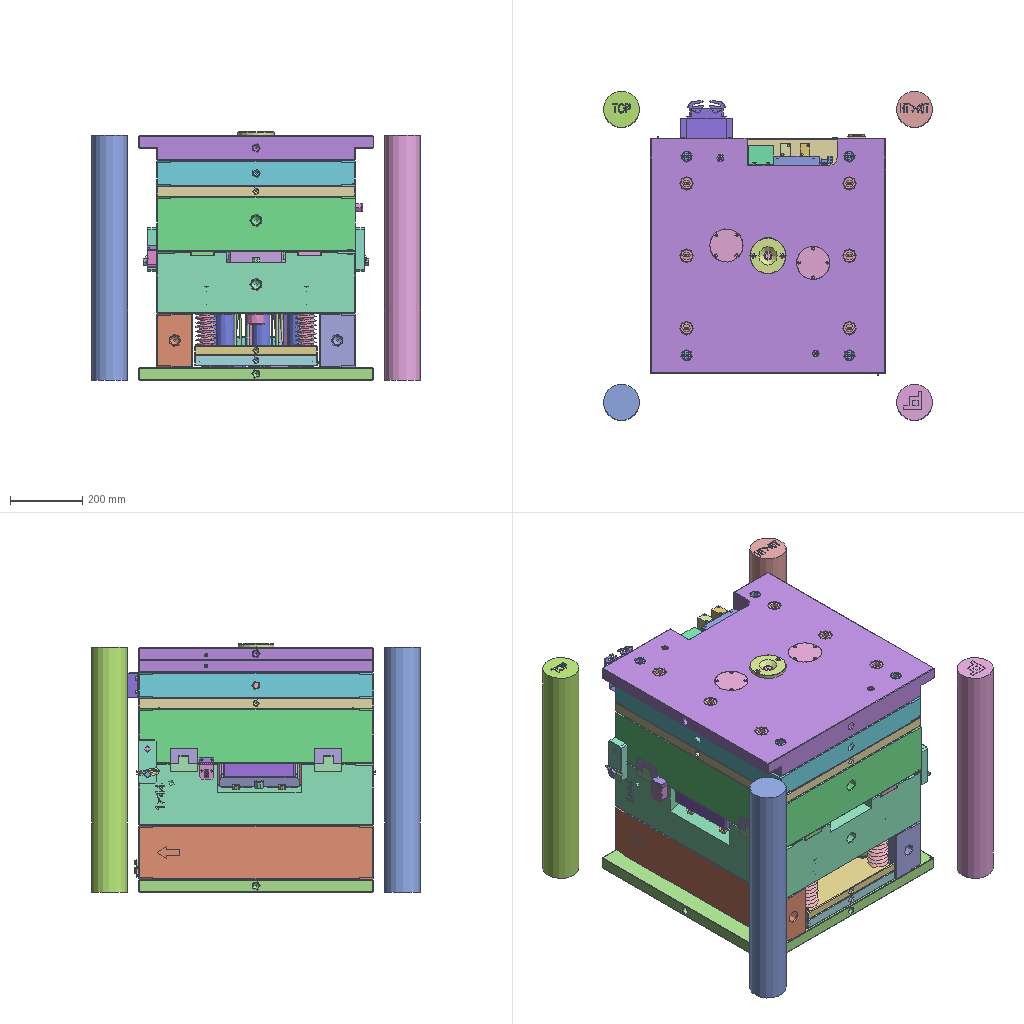Assembly | STEP file | 222 different items | 769 placed | box 910 x 908 x 687 mm
Parts list (item | name | quantity | parent item | size | volume):
1 | Tie Bars 360T | x1 | in 4-Mark_FACET | 910 x 910 x 677 mm | 21266346 mm3
2 | P011002M004-000 | x1 | in 3.1-Core_MODEL | 14.13 x 12.392 x 104.223 mm | 11432 mm3
3 | P011002M001-000 | x1 | in 3.1-Core_MODEL | - | 8732040 mm3
4 | P011002M003-000 | x1 | in 3.1-Core_MODEL | 12.084 x 12.031 x 102.825 mm | 9089 mm3
5 | P011002M005-000 | x1 | in 3.1-Core_MODEL | 67.862 x 16 x 35.33 mm | 24834 mm3
6 | P011002M006-000 | x1 | in 3.1-Core_MODEL | 70.25 x 27 x 35.42 mm | 49386 mm3
7 | P011002M008-000 | x1 | in 3.1-Core_MODEL | 73.5 x 17 x 37.933 mm | 27742 mm3
8 | P011002M009-000 | x1 | in 3.1-Core_MODEL | 73.5 x 19 x 37.504 mm | 38643 mm3
9 | P011002M007-000 | x1 | in 3.1-Core_MODEL | 72.03 x 27.74 x 35.47 mm | 32998 mm3
10 | P011002M002-000 | x1 | in 3.1-Core_MODEL | 110.341 x 214.577 x 105.416 mm | 1490799 mm3
11 | EM10503500 | x12 | in 3.1-Core_MODEL, 3.3.6-Lifter 06_MODEL, 3.3.3-Lifter 03_MODEL, 3.3.4-Lifter 04_MODEL, 3.3.5-Lifter 05_MODEL | 8.5 x 8.5 x 40 mm | 920.076 mm3
12 | EM11211000 | x11 | in 3.1-Core_MODEL | 18 x 18 x 122 mm | 14775 mm3
13 | P011002M012-000 | x1 | in 3.1-Core_MODEL | 16.594 x 32.5 x 39.15 mm | 15176 mm3
14 | EM10606000 | x1 | in 3.1-Core_MODEL | 10 x 10 x 66 mm | 2076 mm3
15 | P011002M013-000 | x1 | in 3.1-Core_MODEL | 17 x 15.5 x 53.228 mm | 4545 mm3
16 | P011002M014-000 | x1 | in 3.1-Core_MODEL | 19 x 16.5 x 58.198 mm | 5006 mm3
17 | P011002M015-000 | x1 | in 3.1-Core_MODEL | 19 x 16.5 x 58.027 mm | 4994 mm3
18 | P011002M011-000 | x1 | in 3.1-Core_MODEL | 10.289 x 8.281 x 94.692 mm | 4991 mm3
19 | P011002M010-000 | x1 | in 3.1-Core_MODEL | 9.465 x 8.201 x 94.193 mm | 4408 mm3
20 | P011002M016-000 | x1 | in 3.1-Core_MODEL | 8.688 x 9.5 x 91.429 mm | 3552 mm3
21 | P011002S001-004 | x1 | in 3.2.1-Slide 01_MODEL | 22 x 82 x 24.22 mm | 33052 mm3
22 | P011002S001-002 | x1 | in 3.2.1-Slide 01_MODEL | 33 x 89.557 x 25 mm | 35725 mm3
23 | P011002S001-003 | x1 | in 3.2.1-Slide 01_MODEL | 22 x 82 x 24.22 mm | 33052 mm3
24 | P011002S001-006 | x1 | in 3.2.1-Slide 01_MODEL | 100 x 50.56 x 14.6 mm | 55263 mm3
25 | P011002S001-007 | x1 | in 3.2.1-Slide 01_MODEL | 20 x 19.153 x 23.411 mm | 6389 mm3
26 | P011002S001-001 | x1 | in 3.2.1-Slide 01_MODEL | 33 x 82.885 x 22 mm | 32044 mm3
27 | P011002S001-000 | x1 | in 3.2.1-Slide 01_MODEL | 120 x 58 x 62.996 mm | 277812 mm3
28 | P011002S001-005 | x1 | in 3.2.1-Slide 01_MODEL | 100 x 15.102 x 35.898 mm | 26958 mm3
29 | EM10802500 | x12 | in 3.2.1-Slide 01_MODEL, 3.2.4-Slide 04_MODEL, 3.3.1-Lifter 01_MODEL, 3.3.2-Lifter 02_MODEL | 13 x 13 x 33 mm | 2154 mm3
30 | EE030603500 | x8 | in 3.2.1-Slide 01_MODEL, 3.2.4-Slide 04_MODEL | 6 x 6 x 37.232 mm | 1919 mm3
31 | SOLID | x58 | in EM10501000 | 8.5 x 8.5 x 15 mm | 429.474 mm3
32 | SOLID | x29 | - | 9.5 x 9.5 x 8 mm | 449.248 mm3
33 | SOLID | x29 | - | 5 x 5 x 12.76 mm | 163.945 mm3
34 | EM10601600 | x39 | in 3.2.1-Slide 01_MODEL, 3.2.2-Slide 02_MODEL, 3.2.3-Slide 03_MODEL, 3.2.4-Slide 04_MODEL, 3.7-Other_MODEL | 10 x 10 x 22 mm | 832.203 mm3
35 | EM10602500 | x20 | in 3.2.1-Slide 01_MODEL, 3.2.2-Slide 02_MODEL, 3.2.3-Slide 03_MODEL, 3.3.1-Lifter 01_MODEL, 3.3.2-Lifter 02_MODEL, 3.3.3-Lifter 03_MODEL, 3.3.5-Lifter 05_MODEL | 10 x 10 x 31 mm | 1087 mm3
36 | EM10803000 | x17 | in 3.2.1-Slide 01_MODEL, 3.2.3-Slide 03_MODEL, 3.2.4-Slide 04_MODEL, 2.2.1-Slide 01_MODEL, 2.2.2-Slide 02_MODEL, 2.2.3-Slide 03_MODEL, 2.2.4-Slide 04_MODEL | 13 x 13 x 38 mm | 2405 mm3
37 | E011204002 | x1 | in 3.2.1-Slide 01_MODEL | - | 1089 mm3
38 | E030603000 | x1 | in 3.2.1-Slide 01_MODEL | 6 x 6 x 32.232 mm | 1637 mm3
39 | P011002S002-000 | x1 | in 3.2.2-Slide 02_MODEL | 70.019 x 220 x 86.547 mm | 835279 mm3
40 | P011002S002-005 | x1 | in 3.2.2-Slide 02_MODEL | 100 x 22 x 65.128 mm | 89552 mm3
41 | P011002S002-002 | x1 | in 3.2.2-Slide 02_MODEL | 103.644 x 32 x 40.64 mm | 72911 mm3
42 | P011002S002-010 | x2 | in 3.2.2-Slide 02_MODEL | 24.439 x 20 x 26.83 mm | 6238 mm3
43 | P011002S002-007 | x1 | in 3.2.2-Slide 02_MODEL | 14.824 x 100 x 40.781 mm | 30059 mm3
44 | P011002S002-003 | x1 | in 3.2.2-Slide 02_MODEL | 94.285 x 31 x 37.408 mm | 61974 mm3
45 | P011002S002-008 | x2 | in 3.2.2-Slide 02_MODEL | 60.486 x 65 x 31.798 mm | 42735 mm3
46 | P011002S002-009 | x1 | in 3.2.2-Slide 02_MODEL | 73.728 x 25 x 55.026 mm | 50035 mm3
47 | P011002S002-004 | x1 | in 3.2.2-Slide 02_MODEL | 100 x 22 x 65.128 mm | 89552 mm3
48 | P011002S002-006 | x1 | in 3.2.2-Slide 02_MODEL | 14.824 x 100 x 40.781 mm | 30059 mm3
49 | P011002S002-001 | x1 | in 3.2.2-Slide 02_MODEL | 113.158 x 33 x 44.092 mm | 87912 mm3
50 | EM10806500 | x2 | in 3.2.2-Slide 02_MODEL | 13 x 13 x 73 mm | 4164 mm3
51 | EE030607000 | x2 | in 3.2.2-Slide 02_MODEL | 6 x 6 x 72.232 mm | 3898 mm3
52 | EM10804500 | x5 | in 3.2.2-Slide 02_MODEL, 2.2.2-Slide 02_MODEL | 13 x 13 x 53 mm | 3159 mm3
53 | EE030606000 | x12 | in 3.2.2-Slide 02_MODEL, 3.2.3-Slide 03_MODEL, 3.3.2-Lifter 02_MODEL | 6 x 6 x 62.232 mm | 3333 mm3
54 | EM10603000 | x6 | in 3.2.2-Slide 02_MODEL, 3.2.4-Slide 04_MODEL, 3.7-Other_MODEL | 10 x 10 x 36 mm | 1228 mm3
55 | EM10804000 | x12 | in 3.2.2-Slide 02_MODEL, 3.2.3-Slide 03_MODEL, 3.7-Other_MODEL, 2.2.3-Slide 03_MODEL | 13 x 13 x 48 mm | 2908 mm3
56 | E011204502 | x6 | in 3.2.2-Slide 02_MODEL, 3.2.3-Slide 03_MODEL, 3.2.4-Slide 04_MODEL | - | 1367 mm3
57 | E030603500 | x6 | in 3.2.2-Slide 02_MODEL, 3.2.3-Slide 03_MODEL, 3.2.4-Slide 04_MODEL | 6 x 6 x 37.232 mm | 1919 mm3
58 | P011002S003-006 | x1 | in 3.2.3-Slide 03_MODEL | 16.561 x 105 x 50.63 mm | 40958 mm3
59 | P011002S003-009 | x1 | in 3.2.3-Slide 03_MODEL | 82.185 x 25 x 53.405 mm | 45412 mm3
60 | P011002S003-005 | x1 | in 3.2.3-Slide 03_MODEL | 100 x 22 x 57.18 mm | 75947 mm3
61 | P011002S003-000 | x1 | in 3.2.3-Slide 03_MODEL | 72.003 x 230 x 92.915 mm | 964495 mm3
62 | P011002S003-007 | x1 | in 3.2.3-Slide 03_MODEL | 16.561 x 105 x 50.63 mm | 40958 mm3
63 | P011002S003-004 | x1 | in 3.2.3-Slide 03_MODEL | 100 x 22 x 57.18 mm | 75947 mm3
64 | P011002S003-001 | x1 | in 3.2.3-Slide 03_MODEL | 113.977 x 32 x 43.155 mm | 84322 mm3
65 | P011002S003-010 | x2 | in 3.2.3-Slide 03_MODEL | 24.439 x 20 x 26.83 mm | 6238 mm3
66 | P011002S003-003 | x1 | in 3.2.3-Slide 03_MODEL | 90.488 x 32 x 36.044 mm | 56970 mm3
67 | P011002S003-008 | x2 | in 3.2.3-Slide 03_MODEL | 60.486 x 82 x 31.798 mm | 54303 mm3
68 | P011002S003-002 | x1 | in 3.2.3-Slide 03_MODEL | 101.347 x 31 x 39.172 mm | 65480 mm3
69 | EM10803500 | x4 | in 3.2.3-Slide 03_MODEL, 3.7-Other_MODEL | 13 x 13 x 43 mm | 2656 mm3
70 | EE030605000 | x2 | in 3.2.3-Slide 03_MODEL | 6 x 6 x 52.232 mm | 2767 mm3
71 | SOLID | x28 | in EM10806000 | 13 x 13 x 68 mm | 3913 mm3
72 | SOLID | x14 | - | 8 x 8 x 21.416 mm | 734.263 mm3
73 | SOLID | x14 | - | 14 x 14 x 55 mm | 4312 mm3
74 | P011002S004-003 | x1 | in 3.2.4-Slide 04_MODEL | 22 x 90 x 22 mm | 37795 mm3
75 | P011002S004-005 | x1 | in 3.2.4-Slide 04_MODEL | 140 x 15.102 x 35.898 mm | 37708 mm3
76 | P011002S004-004 | x1 | in 3.2.4-Slide 04_MODEL | 22 x 90 x 22 mm | 37795 mm3
77 | P011002S004-002 | x1 | in 3.2.4-Slide 04_MODEL | 26 x 79.009 x 22.435 mm | 34276 mm3
78 | P011002S004-000 | x1 | in 3.2.4-Slide 04_MODEL | 162 x 60 x 77 mm | 547857 mm3
79 | P011002S004-007 | x1 | in 3.2.4-Slide 04_MODEL | 20 x 18 x 25 mm | 7143 mm3
80 | P011002S004-001 | x1 | in 3.2.4-Slide 04_MODEL | 29 x 101.051 x 22.958 mm | 42473 mm3
81 | P011002S004-006 | x1 | in 3.2.4-Slide 04_MODEL | 142 x 55 x 12 mm | 88183 mm3
82 | P011002L006-000 | x1 | in 3.3.6-Lifter 06_MODEL | 25 x 8.891 x 318.622 mm | 57302 mm3
83 | P011002L001-000 | x1 | in 3.3.1-Lifter 01_MODEL | 38.903 x 161.923 x 102.441 mm | 296499 mm3
84 | P011002L001-005 | x4 | in 3.3.1-Lifter 01_MODEL | 29.573 x 4.8 x 27.272 mm | 1761 mm3
85 | P011002L001-004 | x2 | in 3.3.1-Lifter 01_MODEL | 36.818 x 34.998 x 27.476 mm | 15941 mm3
86 | P011002L001-003 | x2 | in 3.3.1-Lifter 01_MODEL | 75 x 68 x 55 mm | 144794 mm3
87 | P011002L001-001 | x2 | in 3.3.1-Lifter 01_MODEL | 43.362 x 16 x 275.795 mm | 48038 mm3
88 | P011002L001-002 | x2 | in 3.3.1-Lifter 01_MODEL | 55 x 25 x 20 mm | 20325 mm3
89 | EE030606500 | x8 | in 3.3.1-Lifter 01_MODEL | 6 x 6 x 67.232 mm | 3615 mm3
90 | SOLID | x8 | in EE060800001 | 12.7 x 12.7 x 2 mm | 149.833 mm3
91 | P011002L001-007 | x1 | in 3.3.1-Lifter 01_MODEL | 8.861 x 29.5 x 8.749 mm | 1779 mm3
92 | P011002L001-006 | x1 | in 3.3.1-Lifter 01_MODEL | 8.861 x 29.5 x 8.749 mm | 1779 mm3
93 | EM40301200 | x4 | in 3.3.1-Lifter 01_MODEL, 3.3.2-Lifter 02_MODEL | 6.84 x 6.84 x 16.272 mm | 238.801 mm3
94 | P011002L002-000 | x1 | in 3.3.2-Lifter 02_MODEL | 38.575 x 161.92 x 99.169 mm | 274542 mm3
95 | P011002L002-002 | x2 | in 3.3.2-Lifter 02_MODEL | 55 x 25 x 20 mm | 20325 mm3
96 | P011002L002-003 | x2 | in 3.3.2-Lifter 02_MODEL | 75 x 68 x 50 mm | 123835 mm3
97 | P011002L002-004 | x2 | in 3.3.2-Lifter 02_MODEL | 36.818 x 34.998 x 27.476 mm | 15941 mm3
98 | P011002L002-005 | x4 | in 3.3.2-Lifter 02_MODEL | 27.634 x 4.8 x 24.553 mm | 1761 mm3
99 | P011002L002-001 | x2 | in 3.3.2-Lifter 02_MODEL | 43.362 x 16 x 275.795 mm | 48288 mm3
100 | EM10805500 | x8 | in 3.3.2-Lifter 02_MODEL | 13 x 13 x 63 mm | 3662 mm3
101 | P011002L002-007 | x1 | in 3.3.2-Lifter 02_MODEL | 8.861 x 29.5 x 8.749 mm | 1779 mm3
102 | P011002L002-006 | x1 | in 3.3.2-Lifter 02_MODEL | 8.861 x 29.5 x 8.749 mm | 1779 mm3
103 | P011002L003-000 | x1 | in 3.3.3-Lifter 03_MODEL | 25 x 7.502 x 312.004 mm | 56592 mm3
104 | P011002L003-001 | x1 | in 3.3.3-Lifter 03_MODEL | 80 x 45 x 20 mm | 57856 mm3
105 | P011002L004-000 | x1 | in 3.3.4-Lifter 04_MODEL | 25 x 7.502 x 311.018 mm | 56283 mm3
106 | P011002L005-000 | x1 | in 3.3.5-Lifter 05_MODEL | 25 x 7.509 x 319.656 mm | 57786 mm3
107 | P011002L005-001 | x1 | in 3.3.5-Lifter 05_MODEL | 100 x 40 x 20 mm | 68887 mm3
108 | 3.4-Cooling System | x2 | in 3-Core Side ASM_MODEL | - | -
109 | E108-07-310 | x1 | in 3.5-Ejector System_TRUE | 13 x 16.5 x 303.697 mm | 15889 mm3
110 | E106-16-310 | x1 | in 3.5-Ejector System_TRUE | 10 x 13 x 301.324 mm | 8818 mm3
111 | E108-10-310 | x1 | in 3.5-Ejector System_TRUE | 13 x 16.5 x 302.023 mm | 15811 mm3
112 | E105-28-315 | x1 | in 3.5-Ejector System_TRUE | 9 x 12 x 309.813 mm | 6362 mm3
113 | E108-12-310 | x1 | in 3.5-Ejector System_TRUE | 13 x 16.5 x 306.86 mm | 16065 mm3
114 | E108-11-315 | x1 | in 3.5-Ejector System_TRUE | 13 x 16.5 x 310.586 mm | 16274 mm3
115 | E108-05-325 | x1 | in 3.5-Ejector System_TRUE | 13 x 16.5 x 321.213 mm | 16796 mm3
116 | E108-03-320 | x1 | in 3.5-Ejector System_TRUE | 13 x 16.5 x 312.703 mm | 16360 mm3
117 | E106-25-315 | x1 | in 3.5-Ejector System_TRUE | 10 x 13 x 312.463 mm | 9128 mm3
118 | E108-15-310 | x1 | in 3.5-Ejector System_TRUE | 13 x 16.5 x 280 mm | 14461 mm3
119 | E106-18-310 | x1 | in 3.5-Ejector System_TRUE | 10 x 13 x 299.38 mm | 8763 mm3
120 | E106-23-315 | x1 | in 3.5-Ejector System_TRUE | 10 x 13 x 307.684 mm | 8994 mm3
121 | E108-14-310 | x1 | in 3.5-Ejector System_TRUE | 13 x 16.5 x 280 mm | 14461 mm3
122 | E106-13-315 | x1 | in 3.5-Ejector System_TRUE | 10 x 13 x 309.676 mm | 9056 mm3
123 | E106-17-310 | x1 | in 3.5-Ejector System_TRUE | 10 x 13 x 302.496 mm | 8853 mm3
124 | E108-04-325 | x1 | in 3.5-Ejector System_TRUE | 13 x 16.5 x 322.523 mm | 16862 mm3
125 | E108-08-310 | x1 | in 3.5-Ejector System_TRUE | 13 x 16.5 x 302.869 mm | 15847 mm3
126 | E106-20-315 | x1 | in 3.5-Ejector System_TRUE | 10 x 13 x 307.336 mm | 8991 mm3
127 | E106-26-325 | x1 | in 3.5-Ejector System_TRUE | 10 x 13 x 318.085 mm | 9301 mm3
128 | E108-06-310 | x1 | in 3.5-Ejector System_TRUE | 13 x 16.5 x 302.992 mm | 15844 mm3
129 | E108-09-310 | x1 | in 3.5-Ejector System_TRUE | 13 x 16.5 x 301.993 mm | 15803 mm3
130 | E105-29-315 | x1 | in 3.5-Ejector System_TRUE | 9 x 12 x 311.151 mm | 6392 mm3
131 | E106-21-315 | x1 | in 3.5-Ejector System_TRUE | 10 x 13 x 308.066 mm | 9009 mm3
132 | E105-27-315 | x1 | in 3.5-Ejector System_TRUE | 9 x 12 x 304.744 mm | 6258 mm3
133 | E105-30-315 | x1 | in 3.5-Ejector System_TRUE | 9 x 12 x 311.08 mm | 6391 mm3
134 | E108-1-312 | x1 | in 3.5-Ejector System_TRUE | 13 x 16.5 x 290 mm | 14963 mm3
135 | E105-19-315 | x1 | in 3.5-Ejector System_TRUE | 9 x 12 x 309.26 mm | 6349 mm3
136 | 3.6-Runner System | x1 | in 3-Core Side ASM_MODEL | - | -
137 | P011002NM05-000 | x1 | in 3.7-Other_MODEL | 65 x 100 x 12 mm | 66526 mm3
138 | P011002NM02-000 | x2 | in 3.7-Other_MODEL | 50 x 85 x 12 mm | 47864 mm3
139 | P011002NM01-000 | x2 | in 3.7-Other_MODEL | 84 x 80 x 12 mm | 69166 mm3
140 | P011002NM03-000 | x2 | in 3.7-Other_MODEL | 35 x 70 x 12 mm | 28000 mm3
141 | P011002NM04-000 | x1 | in 3.7-Other_MODEL | 65 x 100 x 12 mm | 66526 mm3
142 | P011002NM06-000 | x1 | in 3.7-Other_MODEL | 31 x 77 x 69 mm | 123856 mm3
143 | P011002NM07-000 | x1 | in 3.7-Other_MODEL | 87 x 31 x 69 mm | 142784 mm3
144 | P011002NM08-000 | x1 | in 3.7-Other_MODEL | 88 x 31 x 69 mm | 144711 mm3
145 | P011002NM09-000 | x1 | in 3.7-Other_MODEL | 31 x 57 x 69 mm | 94738 mm3
146 | EM11007500 | x7 | in 3.7-Other_MODEL | 16 x 16 x 85 mm | 7551 mm3
147 | P011002NM10-000 | x3 | in 3.7-Other_MODEL | 35 x 35 x 38 mm | 32907 mm3
148 | P011002NM12-000 | x7 | in 3.7-Other_MODEL | 50 x 50 x 150 mm | 291723 mm3
149 | P011002NM11-000 | x2 | in 3.7-Other_MODEL | 40 x 40 x 150 mm | 185820 mm3
150 | P011002NM13-000 | x2 | in 3.7-Other_MODEL | 50 x 50 x 30 mm | 55572 mm3
151 | P011002NM14-000 | x1 | in 3.7-Other_MODEL | 150 x 50 x 25 mm | 168344 mm3
152 | P011002NM16-000 | x1 | in 3.7-Other_MODEL | 50 x 5 x 49 mm | 10135 mm3
153 | P011002NM15-000 | x1 | in 3.7-Other_MODEL | 30 x 5 x 50 mm | 7166 mm3
154 | E112002500 | x4 | in 3.7-Other_MODEL | 20 x 20 x 20 mm | 6268 mm3
155 | E016017503 | x4 | in 3.7-Other_MODEL | - | 163409 mm3
156 | PH15012004 | x2 | in 3.7-Other_MODEL | 65.87 x 120 x 90.403 mm | 187828 mm3
157 | EM11204000 | x9 | in 3.7-Other_MODEL | 18 x 18 x 52 mm | 6858 mm3
158 | EM10301400 | x2 | in 3.7-Other_MODEL | 5 x 5 x 17 mm | 149.174 mm3
159 | EM10401000 | x2 | in 3.7-Other_MODEL | 7 x 7 x 14 mm | 262.339 mm3
160 | EN80200001 | x1 | in 3.7-Other_MODEL | 21 x 20.3 x 18.187 mm | 1904 mm3
161 | E050000001 | x1 | in 3.7-Other_MODEL | 26.859 x 11 x 37.801 mm | 4792 mm3
162 | EM10601400 | x2 | in 3.7-Other_MODEL | 10 x 10 x 20 mm | 775.654 mm3
163 | E042000001 | x1 | in 3.7-Other_MODEL | 38 x 60 x 38.607 mm | 56849 mm3
164 | D17XH8Xd12XA6XB8X310LXN180 | x1 | in 3.7-Other_MODEL | 15.5 x 17 x 309.851 mm | 27016 mm3
165 | P011002B001-000 | x1 | in 3.8-Mold base_MODEL | - | 41496641 mm3
166 | P011002C002-000 | x2 | in P011002C001-000_MODEL, 3.8-Mold base_MODEL | 100 x 650 x 150 mm | 9316840 mm3
167 | SOLID | x1 | in P011002C001-000_MODEL | 100 x 650 x 150 mm | 9243091 mm3
168 | P011002B004-000 | x1 | in 3.8-Mold base_MODEL | 650 x 650 x 35 mm | 13284442 mm3
169 | RP-D30-287L | x4 | in 3.8-Mold base_MODEL | 36 x 36 x 287 mm | 205979 mm3
170 | P011002B003-000 | x1 | in 3.8-Mold base_MODEL | 340 x 650 x 30 mm | 5385169 mm3
171 | P011002B002-000 | x1 | in 3.8-Mold base_MODEL | 340 x 650 x 25 mm | 4617723 mm3
172 | LKM-Top Locks-TOP_75-B | x4 | in 3.8-Mold base_MODEL | 30 x 75 x 51.5 mm | 60575 mm3
173 | DP20-1 | x8 | in 3.8-Mold base_MODEL | 20 x 20 x 71.774 mm | 40454 mm3
174 | M24-1 | x6 | in 3.8-Mold base_MODEL | 36 x 36 x 214 mm | 107145 mm3
175 | M16-2 | x8 | in 3.8-Mold base_MODEL | 24 x 24 x 56 mm | 13524 mm3
176 | GP50 | x4 | in 3.8-Mold base_MODEL | 58 x 58 x 310 mm | 612293 mm3
177 | EGP | x4 | in 3.8-Mold base_MODEL | 45 x 45 x 220 mm | 186041 mm3
178 | STP | x14 | in 3.8-Mold base_MODEL | 28 x 28 x 12.4 mm | 3112 mm3
179 | M12-1 | x8 | in 3.8-Mold base_MODEL | 18 x 18 x 47 mm | 6292 mm3
180 | P011002F001-000 | x1 | in 2.1-Cavity_MODEL | - | 7659861 mm3
181 | EM11207000 | x8 | in 2.1-Cavity_MODEL | 18 x 18 x 82 mm | 10251 mm3
182 | P011002S001-008 | x1 | in 2.2.1-Slide 01_MODEL | 25 x 35.334 x 83.861 mm | 28077 mm3
183 | P011002S001-009 | x1 | in 2.2.1-Slide 01_MODEL | 100 x 85 x 70 mm | 323771 mm3
184 | EM10807500 | x2 | in 2.2.1-Slide 01_MODEL | 13 x 13 x 83 mm | 4667 mm3
185 | P011002S002-011 | x2 | in 2.2.2-Slide 02_MODEL | 34.904 x 25 x 99.124 mm | 32836 mm3
186 | P011002S002-012 | x1 | in 2.2.2-Slide 02_MODEL | 110 x 190 x 78 mm | 738525 mm3
187 | P011002S003-011 | x2 | in 2.2.3-Slide 03_MODEL | 36.296 x 25 x 109.027 mm | 35448 mm3
188 | P011002S003-012 | x1 | in 2.2.3-Slide 03_MODEL | 110 x 200 x 90 mm | 805824 mm3
189 | P011002S004-008 | x2 | in 2.2.4-Slide 04_MODEL | 20 x 32.087 x 88.754 mm | 18799 mm3
190 | P011002S004-009 | x1 | in 2.2.4-Slide 04_MODEL | 135 x 40 x 25 mm | 110970 mm3
191 | 2.3-Lifter | x1 | in 2-Cavity Side ASM_MODEL | - | -
192 | SOLID | x22 | in EM3380000 | 16.662 x 16.662 x 12.01 mm | 2091 mm3
193 | SOLID | x11 | - | 16.662 x 16.662 x 12.01 mm | 1384 mm3
194 | EN53801200 | x4 | in CO-FC-01_MODEL, CO-FC-02_MODEL | 22 x 24.249 x 32.01 mm | 7856 mm3
195 | EC21600001 | x4 | in CO-FC-01_MODEL, CO-FC-02_MODEL | 22.4 x 22.4 x 1.8 mm | 613.838 mm3
196 | SOLID | x1 | in CO-FC-01_MODEL | 356 x 182.01 x 78 mm | 174730 mm3
197 | EC31200008 | x1 | in CO-FC-02_MODEL | 12 x 12 x 12 mm | 1282 mm3
198 | SOLID | x1 | in CO-FC-02_MODEL | 440 x 197.312 x 76 mm | 258377 mm3
199 | 2.5-Ejector System | x1 | in 2-Cavity Side ASM_MODEL | - | -
200 | EM31800001 | x4 | in 2.6-Runner System_MODEL | 9.728 x 9.728 x 8.365 mm | 484.697 mm3
201 | EM10503000 | x4 | in 2.6-Runner System_MODEL | 9.5 x 9.5 x 40.261 mm | 1873 mm3
202 | M10600800 | x4 | in 2.6-Runner System_MODEL | 10 x 10 x 24.812 mm | 985.086 mm3
203 | COMPOUND | x1 | in 2.6-Runner System_MODEL | 514.266 x 513.429 x 330.33 mm | 7966584 mm3
204 | P011002NF02-000 | x3 | in 2.7-Other_MODEL | 80 x 31 x 84 mm | 154459 mm3
205 | P011002NF03-000 | x1 | in 2.7-Other_MODEL | 31 x 60 x 84 mm | 108643 mm3
206 | EM11009000 | x8 | in 2.7-Other_MODEL | 16 x 16 x 100 mm | 8729 mm3
207 | P011002NF01-000 | x1 | in 2.7-Other_MODEL | 100 x 100 x 18 mm | 119839 mm3
208 | EM10802000 | x2 | in 2.7-Other_MODEL | 13 x 13 x 28 mm | 1902 mm3
209 | EM40500800 | x6 | in 2.7-Other_MODEL | 11.4 x 11.4 x 17.76 mm | 658.01 mm3
210 | P011002NF05-000 | x1 | in 2.7-Other_MODEL | 75 x 192.5 x 5 mm | 70540 mm3
211 | P011002NF04-000 | x1 | in 2.7-Other_MODEL | 190 x 75 x 5 mm | 70407 mm3
212 | P011002A003-000 | x1 | in 2.8-Mold base_MODEL | 550 x 650 x 70 mm | 18968143 mm3
213 | P011002A002-000 | x1 | in 2.8-Mold base_MODEL | 550 x 650 x 30 mm | 10420877 mm3
214 | P011002A004-000 | x1 | in 2.8-Mold base_MODEL | 650 x 650 x 70 mm | 24694977 mm3
215 | P011002A001-000 | x1 | in 2.8-Mold base_MODEL | 550 x 650 x 150 mm | 35811112 mm3
216 | M24-2 | x6 | in 2.8-Mold base_MODEL | 36 x 36 x 204 mm | 102621 mm3
217 | M20-1 | x4 | in 2.8-Mold base_MODEL | 30 x 30 x 100 mm | 36177 mm3
218 | M16-1 | x4 | in 2.8-Mold base_MODEL | 24 x 24 x 96 mm | 21566 mm3
219 | DP20X210 | x2 | in 2.8-Mold base_MODEL | 20 x 20 x 210 mm | 65178 mm3
220 | LKM-Top Locks-TOP_75-A | x4 | in 2.8-Mold base_MODEL | 30 x 75 x 51.5 mm | 70556 mm3
221 | GB-D50-150L | x4 | in 2.8-Mold base_MODEL | 76 x 76 x 150 mm | 293063 mm3
222 | 20110925@CORE-RH | x1 | in 1-Product_FACET | 186.272 x 292.181 x 109.099 mm | 237694 mm3
Placements (level | parent | child | x y z in mm | rotation matrix by rows), first 285 of 914 lines:
1 | subassembly 2 | 4-Mark_FACET | 0.0 0.0 0.0 | 1 0 0 0 1 0 0 0 1
2 | 4-Mark_FACET | Tie Bars 360T | 0.0 0.0 0.0 | 1 0 0 0 1 0 0 0 1
1 | subassembly 2 | 3-Core Side ASM_MODEL | 0.0 0.0 0.0 | 1 0 0 0 1 0 0 0 1
2 | 3-Core Side ASM_MODEL | 3.1-Core_MODEL | 0.0 0.0 0.0 | 1 0 0 0 1 0 0 0 1
3 | 3.1-Core_MODEL | P011002M004-000 | 0.0 0.0 0.0 | 1 0 0 0 1 0 0 0 1
3 | 3.1-Core_MODEL | P011002M001-000 | 0.0 0.0 0.0 | 1 0 0 0 1 0 0 0 1
3 | 3.1-Core_MODEL | P011002M003-000 | 0.0 0.0 0.0 | 1 0 0 0 1 0 0 0 1
3 | 3.1-Core_MODEL | P011002M005-000 | 0.0 0.0 0.0 | 1 0 0 0 1 0 0 0 1
3 | 3.1-Core_MODEL | P011002M006-000 | 0.0 0.0 0.0 | 1 0 0 0 1 0 0 0 1
3 | 3.1-Core_MODEL | P011002M008-000 | 0.0 0.0 0.0 | 1 0 0 0 1 0 0 0 1
3 | 3.1-Core_MODEL | P011002M009-000 | 0.0 0.0 0.0 | 1 0 0 0 1 0 0 0 1
3 | 3.1-Core_MODEL | P011002M007-000 | 0.0 0.0 0.0 | 1 0 0 0 1 0 0 0 1
3 | 3.1-Core_MODEL | P011002M002-000 | 0.0 0.0 0.0 | 1 0 0 0 1 0 0 0 1
3 | 3.1-Core_MODEL | EM10503500 | -129.932 40.02 37.0 | 1 0 0 0 1 0 0 0 1
3 | 3.1-Core_MODEL | EM10503500 | 107.019 -21.406 27.0 | 1 0 0 0 1 0 0 0 1
3 | 3.1-Core_MODEL | EM10503500 | 144.019 -21.406 27.0 | 1 0 0 0 1 0 0 0 1
3 | 3.1-Core_MODEL | EM10503500 | -108.932 42.02 37.0 | 1 0 0 0 1 0 0 0 1
3 | 3.1-Core_MODEL | EM11211000 | -15.0 12.0 -151.0 | -1 0 0 0 1 0 0 0 -1
3 | 3.1-Core_MODEL | EM11211000 | 145.0 -180.0 -151.0 | -1 0 0 0 1 0 0 0 -1
3 | 3.1-Core_MODEL | EM11211000 | 20.0 -38.0 -151.0 | -1 0 0 0 1 0 0 0 -1
3 | 3.1-Core_MODEL | EM11211000 | -15.0 -68.0 -151.0 | -1 0 0 0 1 0 0 0 -1
3 | 3.1-Core_MODEL | EM11211000 | -145.0 180.0 -151.0 | -1 0 0 0 1 0 0 0 -1
3 | 3.1-Core_MODEL | EM11211000 | 20.0 52.0 -151.0 | -1 0 0 0 1 0 0 0 -1
3 | 3.1-Core_MODEL | EM11211000 | -145.0 20.0 -151.0 | -1 0 0 0 1 0 0 0 -1
3 | 3.1-Core_MODEL | EM11211000 | 145.0 45.0 -151.0 | -1 0 0 0 1 0 0 0 -1
3 | 3.1-Core_MODEL | EM11211000 | 145.0 180.0 -151.0 | -1 0 0 0 1 0 0 0 -1
3 | 3.1-Core_MODEL | EM11211000 | -15.0 77.0 -151.0 | -1 0 0 0 1 0 0 0 -1
3 | 3.1-Core_MODEL | EM11211000 | -145.0 -180.0 -151.0 | -1 0 0 0 1 0 0 0 -1
3 | 3.1-Core_MODEL | P011002M012-000 | 0.0 0.0 0.0 | 1 0 0 0 1 0 0 0 1
3 | 3.1-Core_MODEL | EM10606000 | -70.0 -4.5 -48.0 | -1 0 0 0 1 0 0 0 -1
3 | 3.1-Core_MODEL | P011002M013-000 | 0.0 0.0 0.0 | 1 0 0 0 1 0 0 0 1
3 | 3.1-Core_MODEL | P011002M014-000 | 0.0 0.0 0.0 | 1 0 0 0 1 0 0 0 1
3 | 3.1-Core_MODEL | P011002M015-000 | 0.0 0.0 0.0 | 1 0 0 0 1 0 0 0 1
3 | 3.1-Core_MODEL | P011002M011-000 | 0.0 0.0 0.0 | 1 0 0 0 1 0 0 0 1
3 | 3.1-Core_MODEL | P011002M010-000 | 0.0 0.0 0.0 | 1 0 0 0 1 0 0 0 1
3 | 3.1-Core_MODEL | P011002M016-000 | 0.0 0.0 0.0 | 1 0 0 0 1 0 0 0 1
2 | 3-Core Side ASM_MODEL | 3.2-Slide_MODEL | 0.0 0.0 0.0 | 1 0 0 0 1 0 0 0 1
3 | 3.2-Slide_MODEL | 3.2.1-Slide 01_MODEL | 0.0 0.0 0.0 | 1 0 0 0 1 0 0 0 1
4 | 3.2.1-Slide 01_MODEL | P011002S001-004 | 0.0 0.0 0.0 | 1 0 0 0 1 0 0 0 1
4 | 3.2.1-Slide 01_MODEL | P011002S001-002 | 0.0 0.0 0.0 | 1 0 0 0 1 0 0 0 1
4 | 3.2.1-Slide 01_MODEL | P011002S001-003 | 0.0 0.0 0.0 | 1 0 0 0 1 0 0 0 1
4 | 3.2.1-Slide 01_MODEL | P011002S001-006 | 0.0 0.0 0.0 | 1 0 0 0 1 0 0 0 1
4 | 3.2.1-Slide 01_MODEL | P011002S001-007 | 0.0 0.0 0.0 | 1 0 0 0 1 0 0 0 1
4 | 3.2.1-Slide 01_MODEL | P011002S001-001 | 0.0 0.0 0.0 | 1 0 0 0 1 0 0 0 1
4 | 3.2.1-Slide 01_MODEL | P011002S001-000 | 0.0 0.0 0.0 | 1 0 0 0 1 0 0 0 1
4 | 3.2.1-Slide 01_MODEL | P011002S001-005 | 0.0 0.0 0.0 | 1 0 0 0 1 0 0 0 1
4 | 3.2.1-Slide 01_MODEL | EM10802500 | -67.5 212.0 19.0 | 1 0 0 0 1 0 0 0 1
4 | 3.2.1-Slide 01_MODEL | EM10802500 | 66.5 212.0 19.0 | 1 0 0 0 1 0 0 0 1
4 | 3.2.1-Slide 01_MODEL | EE030603500 | 66.5 230.0 19.0 | 1 0 0 0 1 0 0 0 1
4 | 3.2.1-Slide 01_MODEL | EM10802500 | -67.5 268.0 19.0 | 1 0 0 0 1 0 0 0 1
4 | 3.2.1-Slide 01_MODEL | EE030603500 | -67.5 249.0 19.0 | 1 0 0 0 1 0 0 0 1
4 | 3.2.1-Slide 01_MODEL | EE030603500 | -67.5 230.0 19.0 | 1 0 0 0 1 0 0 0 1
4 | 3.2.1-Slide 01_MODEL | EM10802500 | 66.5 268.0 19.0 | 1 0 0 0 1 0 0 0 1
4 | 3.2.1-Slide 01_MODEL | EE030603500 | 66.5 249.0 19.0 | 1 0 0 0 1 0 0 0 1
4 | 3.2.1-Slide 01_MODEL | EM10501000 | 34.5 253.791 26.161 | 0 1 0 -0.2079 0 0.9781 0.9781 0 0.2079
5 | EM10501000 | SOLID | 0.0 0.0 0.0 | 1 0 0 0 1 0 0 0 1
5 | EM10501000 | subassembly 1 | 0.0 0.0 0.0 | 1 0 0 0 1 0 0 0 1
6 | subassembly 1 | SOLID | 0.0 0.0 0.0 | 1 0 0 0 1 0 0 0 1
6 | subassembly 1 | SOLID | 0.0 0.0 0.0 | 1 0 0 0 1 0 0 0 1
6 | subassembly 1 | SOLID | 0.0 0.0 0.0 | 1 0 0 0 1 0 0 0 1
4 | 3.2.1-Slide 01_MODEL | EM10501000 | -35.5 253.791 26.161 | 0 1 0 -0.2079 0 0.9781 0.9781 0 0.2079
5 | EM10501000 | SOLID | 0.0 0.0 0.0 | 1 0 0 0 1 0 0 0 1
5 | EM10501000 | subassembly 1 | 0.0 0.0 0.0 | 1 0 0 0 1 0 0 0 1
6 | subassembly 1 | SOLID | 0.0 0.0 0.0 | 1 0 0 0 1 0 0 0 1
6 | subassembly 1 | SOLID | 0.0 0.0 0.0 | 1 0 0 0 1 0 0 0 1
6 | subassembly 1 | SOLID | 0.0 0.0 0.0 | 1 0 0 0 1 0 0 0 1
4 | 3.2.1-Slide 01_MODEL | EM10601600 | -35.5 255.167 -11.891 | 0 -1 0 0.9986 0 0.05234 -0.05234 0 0.9986
4 | 3.2.1-Slide 01_MODEL | EM10601600 | -35.5 225.208 -10.321 | 0 -1 0 0.9986 0 0.05234 -0.05234 0 0.9986
4 | 3.2.1-Slide 01_MODEL | EM10601600 | 34.5 225.208 -10.321 | 0 -1 0 0.9986 0 0.05234 -0.05234 0 0.9986
4 | 3.2.1-Slide 01_MODEL | EM10601600 | 34.5 255.167 -11.891 | 0 -1 0 0.9986 0 0.05234 -0.05234 0 0.9986
4 | 3.2.1-Slide 01_MODEL | EM10602500 | -0.5 274.69 -2.4 | 0 -1 0 0.9986 0 0.05234 -0.05234 0 0.9986
4 | 3.2.1-Slide 01_MODEL | EM10803000 | -33.5 210.0 50.0 | 0 -1 0 0.9986 0 0.05234 -0.05234 0 0.9986
4 | 3.2.1-Slide 01_MODEL | EM10803000 | 31.5 210.0 46.0 | 0 -1 0 0.9986 0 0.05234 -0.05234 0 0.9986
4 | 3.2.1-Slide 01_MODEL | E011204002 | -0.5 214.979 0.215 | 0 1 0 -0.05234 0 -0.9986 -0.9986 0 0.05234
4 | 3.2.1-Slide 01_MODEL | E030603000 | -0.5 212.982 0.3196 | 0 1 0 0.05234 0 0.9986 0.9986 0 -0.05234
3 | 3.2-Slide_MODEL | 3.2.2-Slide 02_MODEL | 0.0 0.0 0.0 | 1 0 0 0 1 0 0 0 1
4 | 3.2.2-Slide 02_MODEL | P011002S002-000 | 0.0 0.0 0.0 | 1 0 0 0 1 0 0 0 1
4 | 3.2.2-Slide 02_MODEL | P011002S002-005 | 0.0 0.0 0.0 | 1 0 0 0 1 0 0 0 1
4 | 3.2.2-Slide 02_MODEL | P011002S002-002 | 0.0 0.0 0.0 | 1 0 0 0 1 0 0 0 1
4 | 3.2.2-Slide 02_MODEL | P011002S002-010 | 0.0 0.0 0.0 | 1 0 0 0 1 0 0 0 1
4 | 3.2.2-Slide 02_MODEL | P011002S002-007 | 0.0 0.0 0.0 | 1 0 0 0 1 0 0 0 1
4 | 3.2.2-Slide 02_MODEL | P011002S002-003 | 0.0 0.0 0.0 | 1 0 0 0 1 0 0 0 1
4 | 3.2.2-Slide 02_MODEL | P011002S002-008 | 0.0 -132.5 0.0 | 1 0 0 0 1 0 0 0 1
4 | 3.2.2-Slide 02_MODEL | P011002S002-009 | 0.0 0.0 0.0 | 1 0 0 0 1 0 0 0 1
4 | 3.2.2-Slide 02_MODEL | P011002S002-008 | 0.0 0.0 0.0 | 1 0 0 0 1 0 0 0 1
4 | 3.2.2-Slide 02_MODEL | P011002S002-004 | 0.0 0.0 0.0 | 1 0 0 0 1 0 0 0 1
4 | 3.2.2-Slide 02_MODEL | P011002S002-010 | 0.0 -132.5 0.0 | 1 0 0 0 1 0 0 0 1
4 | 3.2.2-Slide 02_MODEL | P011002S002-006 | 0.0 0.0 0.0 | 1 0 0 0 1 0 0 0 1
4 | 3.2.2-Slide 02_MODEL | P011002S002-001 | 0.0 0.0 0.0 | 1 0 0 0 1 0 0 0 1
4 | 3.2.2-Slide 02_MODEL | EM10806500 | 235.0 -102.0 19.0 | 1 0 0 0 1 0 0 0 1
4 | 3.2.2-Slide 02_MODEL | EE030607000 | 217.0 -102.0 19.0 | 1 0 0 0 1 0 0 0 1
4 | 3.2.2-Slide 02_MODEL | EM10804500 | 177.0 132.0 19.0 | 1 0 0 0 1 0 0 0 1
4 | 3.2.2-Slide 02_MODEL | EE030607000 | 217.0 132.0 19.0 | 1 0 0 0 1 0 0 0 1
4 | 3.2.2-Slide 02_MODEL | EE030606000 | 197.0 132.0 19.0 | 1 0 0 0 1 0 0 0 1
4 | 3.2.2-Slide 02_MODEL | EE030606000 | 197.0 -102.0 19.0 | 1 0 0 0 1 0 0 0 1
4 | 3.2.2-Slide 02_MODEL | EM10804500 | 177.0 -102.0 19.0 | 1 0 0 0 1 0 0 0 1
4 | 3.2.2-Slide 02_MODEL | EM10806500 | 235.0 132.0 19.0 | 1 0 0 0 1 0 0 0 1
4 | 3.2.2-Slide 02_MODEL | EM10501000 | 232.465 -75.0 -3.455 | -0.1736 0 0.9848 0 -1 0 0.9848 0 0.1736
5 | EM10501000 | SOLID | 0.0 0.0 0.0 | 1 0 0 0 1 0 0 0 1
5 | EM10501000 | subassembly 1 | 0.0 0.0 0.0 | 1 0 0 0 1 0 0 0 1
6 | subassembly 1 | SOLID | 0.0 0.0 0.0 | 1 0 0 0 1 0 0 0 1
6 | subassembly 1 | SOLID | 0.0 0.0 0.0 | 1 0 0 0 1 0 0 0 1
6 | subassembly 1 | SOLID | 0.0 0.0 0.0 | 1 0 0 0 1 0 0 0 1
4 | 3.2.2-Slide 02_MODEL | EM10501000 | 228.992 -75.0 16.241 | -0.1736 0 0.9848 0 -1 0 0.9848 0 0.1736
5 | EM10501000 | SOLID | 0.0 0.0 0.0 | 1 0 0 0 1 0 0 0 1
5 | EM10501000 | subassembly 1 | 0.0 0.0 0.0 | 1 0 0 0 1 0 0 0 1
6 | subassembly 1 | SOLID | 0.0 0.0 0.0 | 1 0 0 0 1 0 0 0 1
6 | subassembly 1 | SOLID | 0.0 0.0 0.0 | 1 0 0 0 1 0 0 0 1
6 | subassembly 1 | SOLID | 0.0 0.0 0.0 | 1 0 0 0 1 0 0 0 1
4 | 3.2.2-Slide 02_MODEL | EM10501000 | 232.465 -0.0 -3.455 | -0.1736 0 0.9848 0 -1 0 0.9848 0 0.1736
5 | EM10501000 | SOLID | 0.0 0.0 0.0 | 1 0 0 0 1 0 0 0 1
5 | EM10501000 | subassembly 1 | 0.0 0.0 0.0 | 1 0 0 0 1 0 0 0 1
6 | subassembly 1 | SOLID | 0.0 0.0 0.0 | 1 0 0 0 1 0 0 0 1
6 | subassembly 1 | SOLID | 0.0 0.0 0.0 | 1 0 0 0 1 0 0 0 1
6 | subassembly 1 | SOLID | 0.0 0.0 0.0 | 1 0 0 0 1 0 0 0 1
4 | 3.2.2-Slide 02_MODEL | EM10501000 | 228.992 -0.0 16.241 | -0.1736 0 0.9848 0 -1 0 0.9848 0 0.1736
5 | EM10501000 | SOLID | 0.0 0.0 0.0 | 1 0 0 0 1 0 0 0 1
5 | EM10501000 | subassembly 1 | 0.0 0.0 0.0 | 1 0 0 0 1 0 0 0 1
6 | subassembly 1 | SOLID | 0.0 0.0 0.0 | 1 0 0 0 1 0 0 0 1
6 | subassembly 1 | SOLID | 0.0 0.0 0.0 | 1 0 0 0 1 0 0 0 1
6 | subassembly 1 | SOLID | 0.0 0.0 0.0 | 1 0 0 0 1 0 0 0 1
4 | 3.2.2-Slide 02_MODEL | EM10501000 | 228.992 30.0 16.241 | -0.1736 0 0.9848 0 -1 0 0.9848 0 0.1736
5 | EM10501000 | SOLID | 0.0 0.0 0.0 | 1 0 0 0 1 0 0 0 1
5 | EM10501000 | subassembly 1 | 0.0 0.0 0.0 | 1 0 0 0 1 0 0 0 1
6 | subassembly 1 | SOLID | 0.0 0.0 0.0 | 1 0 0 0 1 0 0 0 1
6 | subassembly 1 | SOLID | 0.0 0.0 0.0 | 1 0 0 0 1 0 0 0 1
6 | subassembly 1 | SOLID | 0.0 0.0 0.0 | 1 0 0 0 1 0 0 0 1
4 | 3.2.2-Slide 02_MODEL | EM10501000 | 232.465 30.0 -3.455 | -0.1736 0 0.9848 0 -1 0 0.9848 0 0.1736
5 | EM10501000 | SOLID | 0.0 0.0 0.0 | 1 0 0 0 1 0 0 0 1
5 | EM10501000 | subassembly 1 | 0.0 0.0 0.0 | 1 0 0 0 1 0 0 0 1
6 | subassembly 1 | SOLID | 0.0 0.0 0.0 | 1 0 0 0 1 0 0 0 1
6 | subassembly 1 | SOLID | 0.0 0.0 0.0 | 1 0 0 0 1 0 0 0 1
6 | subassembly 1 | SOLID | 0.0 0.0 0.0 | 1 0 0 0 1 0 0 0 1
4 | 3.2.2-Slide 02_MODEL | EM10501000 | 232.465 105.0 -3.455 | -0.1736 0 0.9848 0 -1 0 0.9848 0 0.1736
5 | EM10501000 | SOLID | 0.0 0.0 0.0 | 1 0 0 0 1 0 0 0 1
5 | EM10501000 | subassembly 1 | 0.0 0.0 0.0 | 1 0 0 0 1 0 0 0 1
6 | subassembly 1 | SOLID | 0.0 0.0 0.0 | 1 0 0 0 1 0 0 0 1
6 | subassembly 1 | SOLID | 0.0 0.0 0.0 | 1 0 0 0 1 0 0 0 1
6 | subassembly 1 | SOLID | 0.0 0.0 0.0 | 1 0 0 0 1 0 0 0 1
4 | 3.2.2-Slide 02_MODEL | EM10501000 | 228.992 105.0 16.241 | -0.1736 0 0.9848 0 -1 0 0.9848 0 0.1736
5 | EM10501000 | SOLID | 0.0 0.0 0.0 | 1 0 0 0 1 0 0 0 1
5 | EM10501000 | subassembly 1 | 0.0 0.0 0.0 | 1 0 0 0 1 0 0 0 1
6 | subassembly 1 | SOLID | 0.0 0.0 0.0 | 1 0 0 0 1 0 0 0 1
6 | subassembly 1 | SOLID | 0.0 0.0 0.0 | 1 0 0 0 1 0 0 0 1
6 | subassembly 1 | SOLID | 0.0 0.0 0.0 | 1 0 0 0 1 0 0 0 1
4 | 3.2.2-Slide 02_MODEL | EM10601600 | 223.261 102.5 -50.205 | 0.9397 0 0.342 0 1 0 -0.342 0 0.9397
4 | 3.2.2-Slide 02_MODEL | EM10601600 | 185.673 102.5 -36.524 | 0.9397 0 0.342 0 1 0 -0.342 0 0.9397
4 | 3.2.2-Slide 02_MODEL | EM10601600 | 223.261 60.0 -50.205 | 0.9397 0 0.342 0 1 0 -0.342 0 0.9397
4 | 3.2.2-Slide 02_MODEL | EM10601600 | 185.673 60.0 -36.524 | 0.9397 0 0.342 0 1 0 -0.342 0 0.9397
4 | 3.2.2-Slide 02_MODEL | EM10601600 | 223.261 -72.5 -50.205 | 0.9397 0 0.342 0 1 0 -0.342 0 0.9397
4 | 3.2.2-Slide 02_MODEL | EM10601600 | 223.261 -30.0 -50.205 | 0.9397 0 0.342 0 1 0 -0.342 0 0.9397
4 | 3.2.2-Slide 02_MODEL | EM10601600 | 185.673 -30.0 -36.524 | 0.9397 0 0.342 0 1 0 -0.342 0 0.9397
4 | 3.2.2-Slide 02_MODEL | EM10601600 | 185.673 -72.5 -36.524 | 0.9397 0 0.342 0 1 0 -0.342 0 0.9397
4 | 3.2.2-Slide 02_MODEL | EM10603000 | 183.794 15.0 -19.878 | 0.9397 0 0.342 0 1 0 -0.342 0 0.9397
4 | 3.2.2-Slide 02_MODEL | EM10603000 | 221.382 15.0 -33.559 | 0.9397 0 0.342 0 1 0 -0.342 0 0.9397
4 | 3.2.2-Slide 02_MODEL | EM10602500 | 244.535 81.25 -47.307 | 0.9397 0 0.342 0 1 0 -0.342 0 0.9397
4 | 3.2.2-Slide 02_MODEL | EM10602500 | 244.535 -51.25 -47.307 | 0.9397 0 0.342 0 1 0 -0.342 0 0.9397
4 | 3.2.2-Slide 02_MODEL | EM10804000 | 220.0 20.0 8.5 | 0 0 1 1 0 0 0 1 0
4 | 3.2.2-Slide 02_MODEL | EM10804000 | 220.0 95.0 8.5 | 0 0 1 1 0 0 0 1 0
4 | 3.2.2-Slide 02_MODEL | EM10804000 | 220.0 -66.0 8.5 | 0 0 1 1 0 0 0 1 0
4 | 3.2.2-Slide 02_MODEL | E011204502 | 183.794 -35.0 -25.84 | -0.342 0 -0.9397 0 -1 0 -0.9397 0 0.342
4 | 3.2.2-Slide 02_MODEL | E030603500 | 181.915 -35.0 -25.156 | 0.342 0 0.9397 0 -1 0 0.9397 0 -0.342
4 | 3.2.2-Slide 02_MODEL | E030603500 | 181.915 65.0 -25.156 | 0.342 0 0.9397 0 -1 0 0.9397 0 -0.342
4 | 3.2.2-Slide 02_MODEL | E011204502 | 183.794 65.0 -25.84 | -0.342 0 -0.9397 0 -1 0 -0.9397 0 0.342
3 | 3.2-Slide_MODEL | 3.2.3-Slide 03_MODEL | 0.0 0.0 0.0 | 1 0 0 0 1 0 0 0 1
4 | 3.2.3-Slide 03_MODEL | P011002S003-006 | 0.0 0.0 0.0 | 1 0 0 0 1 0 0 0 1
4 | 3.2.3-Slide 03_MODEL | P011002S003-009 | 0.0 0.0 0.0 | 1 0 0 0 1 0 0 0 1
4 | 3.2.3-Slide 03_MODEL | P011002S003-005 | 0.0 0.0 0.0 | 1 0 0 0 1 0 0 0 1
4 | 3.2.3-Slide 03_MODEL | P011002S003-000 | 0.0 0.0 0.0 | 1 0 0 0 1 0 0 0 1
4 | 3.2.3-Slide 03_MODEL | P011002S003-007 | 0.0 0.0 0.0 | 1 0 0 0 1 0 0 0 1
4 | 3.2.3-Slide 03_MODEL | P011002S003-004 | 0.0 0.0 0.0 | 1 0 0 0 1 0 0 0 1
4 | 3.2.3-Slide 03_MODEL | P011002S003-001 | 0.0 0.0 0.0 | 1 0 0 0 1 0 0 0 1
4 | 3.2.3-Slide 03_MODEL | P011002S003-010 | 0.0 -127.0 0.0 | 1 0 0 0 1 0 0 0 1
4 | 3.2.3-Slide 03_MODEL | P011002S003-003 | 0.0 0.0 0.0 | 1 0 0 0 1 0 0 0 1
4 | 3.2.3-Slide 03_MODEL | P011002S003-008 | 0.0 0.0 0.0 | 1 0 0 0 1 0 0 0 1
4 | 3.2.3-Slide 03_MODEL | P011002S003-008 | 0.0 -127.0 0.0 | 1 0 0 0 1 0 0 0 1
4 | 3.2.3-Slide 03_MODEL | P011002S003-002 | 0.0 0.0 0.0 | 1 0 0 0 1 0 0 0 1
4 | 3.2.3-Slide 03_MODEL | P011002S003-010 | 0.0 0.0 0.0 | 1 0 0 0 1 0 0 0 1
4 | 3.2.3-Slide 03_MODEL | EE030606000 | -217.0 -131.0 19.0 | 1 0 0 0 1 0 0 0 1
4 | 3.2.3-Slide 03_MODEL | EM10803500 | -177.0 -131.0 19.0 | 1 0 0 0 1 0 0 0 1
4 | 3.2.3-Slide 03_MODEL | EE030605000 | -197.0 113.0 19.0 | 1 0 0 0 1 0 0 0 1
4 | 3.2.3-Slide 03_MODEL | EE030605000 | -197.0 -131.0 19.0 | 1 0 0 0 1 0 0 0 1
4 | 3.2.3-Slide 03_MODEL | EM10806000 | -237.0 -131.0 19.0 | 1 0 0 0 1 0 0 0 1
5 | EM10806000 | SOLID | 0.0 0.0 0.0 | 1 0 0 0 1 0 0 0 1
5 | EM10806000 | subassembly 1 | 0.0 0.0 0.0 | 1 0 0 0 1 0 0 0 1
6 | subassembly 1 | SOLID | 0.0 0.0 0.0 | 1 0 0 0 1 0 0 0 1
6 | subassembly 1 | SOLID | 0.0 0.0 0.0 | 1 0 0 0 1 0 0 0 1
6 | subassembly 1 | SOLID | 0.0 0.0 0.0 | 1 0 0 0 1 0 0 0 1
4 | 3.2.3-Slide 03_MODEL | EM10803500 | -177.0 113.0 19.0 | 1 0 0 0 1 0 0 0 1
4 | 3.2.3-Slide 03_MODEL | EM10806000 | -237.0 113.0 19.0 | 1 0 0 0 1 0 0 0 1
5 | EM10806000 | SOLID | 0.0 0.0 0.0 | 1 0 0 0 1 0 0 0 1
5 | EM10806000 | subassembly 1 | 0.0 0.0 0.0 | 1 0 0 0 1 0 0 0 1
6 | subassembly 1 | SOLID | 0.0 0.0 0.0 | 1 0 0 0 1 0 0 0 1
6 | subassembly 1 | SOLID | 0.0 0.0 0.0 | 1 0 0 0 1 0 0 0 1
6 | subassembly 1 | SOLID | 0.0 0.0 0.0 | 1 0 0 0 1 0 0 0 1
4 | 3.2.3-Slide 03_MODEL | EE030606000 | -217.0 113.0 19.0 | 1 0 0 0 1 0 0 0 1
4 | 3.2.3-Slide 03_MODEL | EM10501000 | -231.57 -24.0 15.619 | -0.1736 0 -0.9848 0 -1 0 -0.9848 0 0.1736
5 | EM10501000 | SOLID | 0.0 0.0 0.0 | 1 0 0 0 1 0 0 0 1
5 | EM10501000 | subassembly 1 | 0.0 0.0 0.0 | 1 0 0 0 1 0 0 0 1
6 | subassembly 1 | SOLID | 0.0 0.0 0.0 | 1 0 0 0 1 0 0 0 1
6 | subassembly 1 | SOLID | 0.0 0.0 0.0 | 1 0 0 0 1 0 0 0 1
6 | subassembly 1 | SOLID | 0.0 0.0 0.0 | 1 0 0 0 1 0 0 0 1
4 | 3.2.3-Slide 03_MODEL | EM10501000 | -231.57 -104.0 15.619 | -0.1736 0 -0.9848 0 -1 0 -0.9848 0 0.1736
5 | EM10501000 | SOLID | 0.0 0.0 0.0 | 1 0 0 0 1 0 0 0 1
5 | EM10501000 | subassembly 1 | 0.0 0.0 0.0 | 1 0 0 0 1 0 0 0 1
6 | subassembly 1 | SOLID | 0.0 0.0 0.0 | 1 0 0 0 1 0 0 0 1
6 | subassembly 1 | SOLID | 0.0 0.0 0.0 | 1 0 0 0 1 0 0 0 1
6 | subassembly 1 | SOLID | 0.0 0.0 0.0 | 1 0 0 0 1 0 0 0 1
4 | 3.2.3-Slide 03_MODEL | EM10501000 | -231.57 6.0 15.619 | -0.1736 0 -0.9848 0 -1 0 -0.9848 0 0.1736
5 | EM10501000 | SOLID | 0.0 0.0 0.0 | 1 0 0 0 1 0 0 0 1
5 | EM10501000 | subassembly 1 | 0.0 0.0 0.0 | 1 0 0 0 1 0 0 0 1
6 | subassembly 1 | SOLID | 0.0 0.0 0.0 | 1 0 0 0 1 0 0 0 1
6 | subassembly 1 | SOLID | 0.0 0.0 0.0 | 1 0 0 0 1 0 0 0 1
6 | subassembly 1 | SOLID | 0.0 0.0 0.0 | 1 0 0 0 1 0 0 0 1
4 | 3.2.3-Slide 03_MODEL | EM10501000 | -231.57 86.0 15.619 | -0.1736 0 -0.9848 0 -1 0 -0.9848 0 0.1736
5 | EM10501000 | SOLID | 0.0 0.0 0.0 | 1 0 0 0 1 0 0 0 1
5 | EM10501000 | subassembly 1 | 0.0 0.0 0.0 | 1 0 0 0 1 0 0 0 1
6 | subassembly 1 | SOLID | 0.0 0.0 0.0 | 1 0 0 0 1 0 0 0 1
6 | subassembly 1 | SOLID | 0.0 0.0 0.0 | 1 0 0 0 1 0 0 0 1
6 | subassembly 1 | SOLID | 0.0 0.0 0.0 | 1 0 0 0 1 0 0 0 1
4 | 3.2.3-Slide 03_MODEL | EM10601600 | -227.959 23.5 -42.915 | 0.9397 0 -0.342 0 1 0 0.342 0 0.9397
4 | 3.2.3-Slide 03_MODEL | EM10601600 | -190.372 23.5 -29.235 | 0.9397 0 -0.342 0 1 0 0.342 0 0.9397
4 | 3.2.3-Slide 03_MODEL | EM10601600 | -190.372 85.5 -29.235 | 0.9397 0 -0.342 0 1 0 0.342 0 0.9397
4 | 3.2.3-Slide 03_MODEL | EM10601600 | -227.959 85.5 -42.915 | 0.9397 0 -0.342 0 1 0 0.342 0 0.9397
4 | 3.2.3-Slide 03_MODEL | EM10601600 | -227.959 -103.5 -42.915 | 0.9397 0 -0.342 0 1 0 0.342 0 0.9397
4 | 3.2.3-Slide 03_MODEL | EM10601600 | -190.372 -103.5 -29.235 | 0.9397 0 -0.342 0 1 0 0.342 0 0.9397
4 | 3.2.3-Slide 03_MODEL | EM10601600 | -190.372 -41.5 -29.235 | 0.9397 0 -0.342 0 1 0 0.342 0 0.9397
4 | 3.2.3-Slide 03_MODEL | EM10601600 | -227.959 -41.5 -42.915 | 0.9397 0 -0.342 0 1 0 0.342 0 0.9397
4 | 3.2.3-Slide 03_MODEL | EM10803000 | -230.779 -9.0 -27.979 | 0.9397 0 -0.342 0 1 0 0.342 0 0.9397
4 | 3.2.3-Slide 03_MODEL | EM10803000 | -183.794 -9.0 -10.878 | 0.9397 0 -0.342 0 1 0 0.342 0 0.9397
4 | 3.2.3-Slide 03_MODEL | EM10602500 | -249.234 54.5 -40.017 | 0.9397 0 -0.342 0 1 0 0.342 0 0.9397
4 | 3.2.3-Slide 03_MODEL | EM10602500 | -249.234 -72.5 -40.017 | 0.9397 0 -0.342 0 1 0 0.342 0 0.9397
4 | 3.2.3-Slide 03_MODEL | EM10804000 | -220.0 -97.0 22.5 | 0 0 -1 -1 0 0 0 1 0
4 | 3.2.3-Slide 03_MODEL | EM10804000 | -220.0 -17.5 22.5 | 0 0 -1 -1 0 0 0 1 0
4 | 3.2.3-Slide 03_MODEL | EM10804000 | -220.0 77.5 22.5 | 0 0 -1 -1 0 0 0 1 0
4 | 3.2.3-Slide 03_MODEL | E030603500 | -181.915 -59.0 -16.156 | 0.342 0 -0.9397 0 -1 0 -0.9397 0 -0.342
4 | 3.2.3-Slide 03_MODEL | E011204502 | -183.794 41.0 -16.84 | -0.342 0 0.9397 0 -1 0 0.9397 0 0.342
4 | 3.2.3-Slide 03_MODEL | E011204502 | -183.794 -59.0 -16.84 | -0.342 0 0.9397 0 -1 0 0.9397 0 0.342
4 | 3.2.3-Slide 03_MODEL | E030603500 | -181.915 41.0 -16.156 | 0.342 0 -0.9397 0 -1 0 -0.9397 0 -0.342
3 | 3.2-Slide_MODEL | 3.2.4-Slide 04_MODEL | 0.0 0.0 0.0 | 1 0 0 0 1 0 0 0 1
4 | 3.2.4-Slide 04_MODEL | P011002S004-003 | 0.0 0.0 0.0 | 1 0 0 0 1 0 0 0 1
4 | 3.2.4-Slide 04_MODEL | P011002S004-005 | 0.0 0.0 0.0 | 1 0 0 0 1 0 0 0 1
4 | 3.2.4-Slide 04_MODEL | P011002S004-004 | 0.0 0.0 0.0 | 1 0 0 0 1 0 0 0 1
4 | 3.2.4-Slide 04_MODEL | P011002S004-002 | 0.0 0.0 0.0 | 1 0 0 0 1 0 0 0 1
4 | 3.2.4-Slide 04_MODEL | P011002S004-000 | 0.0 0.0 0.0 | 1 0 0 0 1 0 0 0 1
4 | 3.2.4-Slide 04_MODEL | P011002S004-007 | 0.0 0.0 0.0 | 1 0 0 0 1 0 0 0 1
4 | 3.2.4-Slide 04_MODEL | P011002S004-001 | 0.0 0.0 0.0 | 1 0 0 0 1 0 0 0 1
4 | 3.2.4-Slide 04_MODEL | P011002S004-006 | 0.0 0.0 0.0 | 1 0 0 0 1 0 0 0 1
4 | 3.2.4-Slide 04_MODEL | EE030603500 | -87.0 -233.0 19.0 | 1 0 0 0 1 0 0 0 1
4 | 3.2.4-Slide 04_MODEL | EE030603500 | 87.0 -257.0 19.0 | 1 0 0 0 1 0 0 0 1
4 | 3.2.4-Slide 04_MODEL | EM10802500 | 87.0 -215.0 19.0 | 1 0 0 0 1 0 0 0 1
4 | 3.2.4-Slide 04_MODEL | EM10802500 | -87.0 -215.0 19.0 | 1 0 0 0 1 0 0 0 1
4 | 3.2.4-Slide 04_MODEL | EE030603500 | -87.0 -257.0 19.0 | 1 0 0 0 1 0 0 0 1
4 | 3.2.4-Slide 04_MODEL | EM10802500 | -87.0 -275.0 19.0 | 1 0 0 0 1 0 0 0 1
4 | 3.2.4-Slide 04_MODEL | EE030603500 | 87.0 -233.0 19.0 | 1 0 0 0 1 0 0 0 1
4 | 3.2.4-Slide 04_MODEL | EM10802500 | 87.0 -275.0 19.0 | 1 0 0 0 1 0 0 0 1
4 | 3.2.4-Slide 04_MODEL | EM10501000 | 42.5 -255.791 41.161 | 0 1 0 -0.2079 0 -0.9781 -0.9781 0 0.2079
5 | EM10501000 | SOLID | 0.0 0.0 0.0 | 1 0 0 0 1 0 0 0 1
5 | EM10501000 | subassembly 1 | 0.0 0.0 0.0 | 1 0 0 0 1 0 0 0 1
6 | subassembly 1 | SOLID | 0.0 0.0 0.0 | 1 0 0 0 1 0 0 0 1
6 | subassembly 1 | SOLID | 0.0 0.0 0.0 | 1 0 0 0 1 0 0 0 1
6 | subassembly 1 | SOLID | 0.0 0.0 0.0 | 1 0 0 0 1 0 0 0 1
4 | 3.2.4-Slide 04_MODEL | EM10501000 | 0.0 -255.791 41.161 | 0 1 0 -0.2079 0 -0.9781 -0.9781 0 0.2079
5 | EM10501000 | SOLID | 0.0 0.0 0.0 | 1 0 0 0 1 0 0 0 1
5 | EM10501000 | subassembly 1 | 0.0 0.0 0.0 | 1 0 0 0 1 0 0 0 1
6 | subassembly 1 | SOLID | 0.0 0.0 0.0 | 1 0 0 0 1 0 0 0 1
6 | subassembly 1 | SOLID | 0.0 0.0 0.0 | 1 0 0 0 1 0 0 0 1
6 | subassembly 1 | SOLID | 0.0 0.0 0.0 | 1 0 0 0 1 0 0 0 1
4 | 3.2.4-Slide 04_MODEL | EM10501000 | -42.5 -255.791 41.161 | 0 1 0 -0.2079 0 -0.9781 -0.9781 0 0.2079
5 | EM10501000 | SOLID | 0.0 0.0 0.0 | 1 0 0 0 1 0 0 0 1
5 | EM10501000 | subassembly 1 | 0.0 0.0 0.0 | 1 0 0 0 1 0 0 0 1
6 | subassembly 1 | SOLID | 0.0 0.0 0.0 | 1 0 0 0 1 0 0 0 1
6 | subassembly 1 | SOLID | 0.0 0.0 0.0 | 1 0 0 0 1 0 0 0 1
6 | subassembly 1 | SOLID | 0.0 0.0 0.0 | 1 0 0 0 1 0 0 0 1
4 | 3.2.4-Slide 04_MODEL | EM10601600 | 56.0 -257.0 -11.0 | 1 0 0 0 1 0 0 0 1
4 | 3.2.4-Slide 04_MODEL | EM10601600 | 56.0 -226.0 -11.0 | 1 0 0 0 1 0 0 0 1
4 | 3.2.4-Slide 04_MODEL | EM10601600 | 0.0 -241.5 -11.0 | 1 0 0 0 1 0 0 0 1
4 | 3.2.4-Slide 04_MODEL | EM10601600 | -56.0 -226.0 -11.0 | 1 0 0 0 1 0 0 0 1
4 | 3.2.4-Slide 04_MODEL | EM10601600 | -56.0 -257.0 -11.0 | 1 0 0 0 1 0 0 0 1
4 | 3.2.4-Slide 04_MODEL | EM10803000 | -52.5 -243.0 46.5 | -1 0 0 0 0 -1 0 -1 0
4 | 3.2.4-Slide 04_MODEL | EM10803000 | 54.5 -245.0 36.5 | -1 0 0 0 0 -1 0 -1 0
4 | 3.2.4-Slide 04_MODEL | EM10603000 | 0.0 -278.0 2.0 | 1 0 0 0 1 0 0 0 1
4 | 3.2.4-Slide 04_MODEL | E011204502 | 40.0 -220.0 1.0 | 1 0 0 0 0 1 0 -1 0
4 | 3.2.4-Slide 04_MODEL | E030603500 | 40.0 -218.0 1.0 | -1 0 0 0 0 -1 0 -1 0
4 | 3.2.4-Slide 04_MODEL | E030603500 | -40.0 -218.0 1.0 | -1 0 0 0 0 -1 0 -1 0